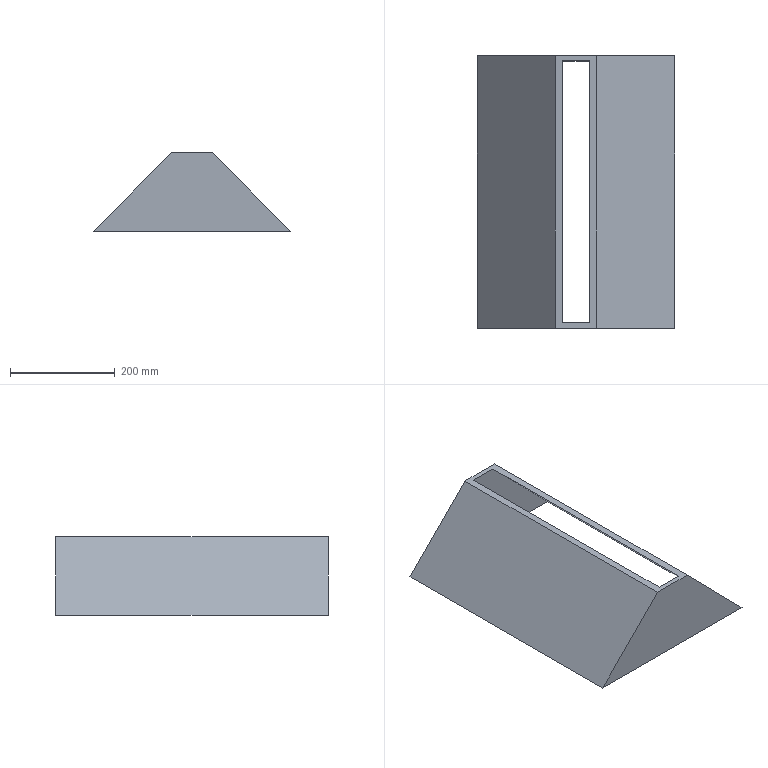Part | SolidWorks | features Extrusion 1, MirrorPattern 1, Shell 1 | 1 solid | 10 faces | box 376 x 520 x 150 mm | volume 2791226 mm3 | plane 10
STEP:
#1=CARTESIAN_POINT('',(-40.,0.,0.));
#2=VERTEX_POINT('',#1);
#3=CARTESIAN_POINT('',(40.,0.,0.));
#4=VERTEX_POINT('',#3);
#5=CARTESIAN_POINT('',(0.,0.,0.));
#6=DIRECTION('',(1.,0.,0.));
#7=VECTOR('',#6,1000.);
#8=LINE('',#5,#7);
#9=EDGE_CURVE('',#2,#4,#8,.T.);
#10=ORIENTED_EDGE('',*,*,#9,.T.);
#11=CARTESIAN_POINT('',(40.,520.,0.));
#12=VERTEX_POINT('',#11);
#13=CARTESIAN_POINT('',(40.,520.,0.));
#14=DIRECTION('',(0.,-1.,0.));
#15=VECTOR('',#14,1000.);
#16=LINE('',#13,#15);
#17=EDGE_CURVE('',#12,#4,#16,.T.);
#18=ORIENTED_EDGE('',*,*,#17,.F.);
#19=CARTESIAN_POINT('',(-40.,520.,0.));
#20=VERTEX_POINT('',#19);
#21=CARTESIAN_POINT('',(0.,520.,0.));
#22=DIRECTION('',(1.,0.,0.));
#23=VECTOR('',#22,1000.);
#24=LINE('',#21,#23);
#25=EDGE_CURVE('',#20,#12,#24,.T.);
#26=ORIENTED_EDGE('',*,*,#25,.F.);
#27=CARTESIAN_POINT('',(-40.,520.,0.));
#28=DIRECTION('',(0.,-1.,0.));
#29=VECTOR('',#28,1000.);
#30=LINE('',#27,#29);
#31=EDGE_CURVE('',#20,#2,#30,.T.);
#32=ORIENTED_EDGE('',*,*,#31,.T.);
#33=EDGE_LOOP('',(#10,#18,#26,#32));
#34=FACE_OUTER_BOUND('',#33,.T.);
#35=CARTESIAN_POINT('',(-25.952,10.,0.));
#36=VERTEX_POINT('',#35);
#37=CARTESIAN_POINT('',(25.952,10.,0.));
#38=VERTEX_POINT('',#37);
#39=CARTESIAN_POINT('',(0.,10.,0.));
#40=DIRECTION('',(1.,0.,0.));
#41=VECTOR('',#40,1000.);
#42=LINE('',#39,#41);
#43=EDGE_CURVE('',#36,#38,#42,.T.);
#44=ORIENTED_EDGE('',*,*,#43,.F.);
#45=CARTESIAN_POINT('',(-25.952,510.,0.));
#46=VERTEX_POINT('',#45);
#47=CARTESIAN_POINT('',(-25.952,520.,0.));
#48=DIRECTION('',(0.,-1.,0.));
#49=VECTOR('',#48,1000.);
#50=LINE('',#47,#49);
#51=EDGE_CURVE('',#46,#36,#50,.T.);
#52=ORIENTED_EDGE('',*,*,#51,.F.);
#53=CARTESIAN_POINT('',(25.952,510.,0.));
#54=VERTEX_POINT('',#53);
#55=CARTESIAN_POINT('',(0.,510.,0.));
#56=DIRECTION('',(1.,0.,0.));
#57=VECTOR('',#56,1000.);
#58=LINE('',#55,#57);
#59=EDGE_CURVE('',#46,#54,#58,.T.);
#60=ORIENTED_EDGE('',*,*,#59,.T.);
#61=CARTESIAN_POINT('',(25.952,520.,0.));
#62=DIRECTION('',(0.,-1.,0.));
#63=VECTOR('',#62,1000.);
#64=LINE('',#61,#63);
#65=EDGE_CURVE('',#54,#38,#64,.T.);
#66=ORIENTED_EDGE('',*,*,#65,.T.);
#67=EDGE_LOOP('',(#44,#52,#60,#66));
#68=FACE_BOUND('',#67,.T.);
#69=CARTESIAN_POINT('',(0.,520.,0.));
#70=DIRECTION('',(0.,0.,-1.));
#71=DIRECTION('',(-1.,0.,0.));
#72=AXIS2_PLACEMENT_3D('',#69,#70,#71);
#73=PLANE('',#72);
#74=ADVANCED_FACE('',(#34,#68),#73,.F.);
#75=CARTESIAN_POINT('',(188.,0.,-150.));
#76=VERTEX_POINT('',#75);
#77=CARTESIAN_POINT('',(-188.,0.,-150.));
#78=VERTEX_POINT('',#77);
#79=CARTESIAN_POINT('',(188.,0.,-150.));
#80=DIRECTION('',(-1.,0.,0.));
#81=VECTOR('',#80,1000.);
#82=LINE('',#79,#81);
#83=EDGE_CURVE('',#76,#78,#82,.T.);
#84=ORIENTED_EDGE('',*,*,#83,.T.);
#85=CARTESIAN_POINT('',(-188.,520.,-150.));
#86=VERTEX_POINT('',#85);
#87=CARTESIAN_POINT('',(-188.,520.,-150.));
#88=DIRECTION('',(0.,-1.,0.));
#89=VECTOR('',#88,1000.);
#90=LINE('',#87,#89);
#91=EDGE_CURVE('',#86,#78,#90,.T.);
#92=ORIENTED_EDGE('',*,*,#91,.F.);
#93=CARTESIAN_POINT('',(188.,520.,-150.));
#94=VERTEX_POINT('',#93);
#95=CARTESIAN_POINT('',(188.,520.,-150.));
#96=DIRECTION('',(-1.,0.,0.));
#97=VECTOR('',#96,1000.);
#98=LINE('',#95,#97);
#99=EDGE_CURVE('',#94,#86,#98,.T.);
#100=ORIENTED_EDGE('',*,*,#99,.F.);
#101=CARTESIAN_POINT('',(188.,520.,-150.));
#102=DIRECTION('',(0.,-1.,0.));
#103=VECTOR('',#102,1000.);
#104=LINE('',#101,#103);
#105=EDGE_CURVE('',#94,#76,#104,.T.);
#106=ORIENTED_EDGE('',*,*,#105,.T.);
#107=EDGE_LOOP('',(#84,#92,#100,#106));
#108=FACE_OUTER_BOUND('',#107,.T.);
#109=CARTESIAN_POINT('',(173.952,10.,-150.));
#110=VERTEX_POINT('',#109);
#111=CARTESIAN_POINT('',(-173.952,10.,-150.));
#112=VERTEX_POINT('',#111);
#113=CARTESIAN_POINT('',(188.,10.,-150.));
#114=DIRECTION('',(-1.,0.,0.));
#115=VECTOR('',#114,1000.);
#116=LINE('',#113,#115);
#117=EDGE_CURVE('',#110,#112,#116,.T.);
#118=ORIENTED_EDGE('',*,*,#117,.F.);
#119=CARTESIAN_POINT('',(173.952,510.,-150.));
#120=VERTEX_POINT('',#119);
#121=CARTESIAN_POINT('',(173.952,520.,-150.));
#122=DIRECTION('',(0.,-1.,0.));
#123=VECTOR('',#122,1000.);
#124=LINE('',#121,#123);
#125=EDGE_CURVE('',#120,#110,#124,.T.);
#126=ORIENTED_EDGE('',*,*,#125,.F.);
#127=CARTESIAN_POINT('',(-173.952,510.,-150.));
#128=VERTEX_POINT('',#127);
#129=CARTESIAN_POINT('',(188.,510.,-150.));
#130=DIRECTION('',(-1.,0.,0.));
#131=VECTOR('',#130,1000.);
#132=LINE('',#129,#131);
#133=EDGE_CURVE('',#120,#128,#132,.T.);
#134=ORIENTED_EDGE('',*,*,#133,.T.);
#135=CARTESIAN_POINT('',(-173.952,520.,-150.));
#136=DIRECTION('',(0.,-1.,0.));
#137=VECTOR('',#136,1000.);
#138=LINE('',#135,#137);
#139=EDGE_CURVE('',#128,#112,#138,.T.);
#140=ORIENTED_EDGE('',*,*,#139,.T.);
#141=EDGE_LOOP('',(#118,#126,#134,#140));
#142=FACE_BOUND('',#141,.T.);
#143=CARTESIAN_POINT('',(188.,520.,-150.));
#144=DIRECTION('',(0.,0.,1.));
#145=DIRECTION('',(1.,0.,0.));
#146=AXIS2_PLACEMENT_3D('',#143,#144,#145);
#147=PLANE('',#146);
#148=ADVANCED_FACE('',(#108,#142),#147,.F.);
#149=CARTESIAN_POINT('',(40.,0.,0.));
#150=DIRECTION('',(0.7023,0.,-0.7118));
#151=VECTOR('',#150,1000.);
#152=LINE('',#149,#151);
#153=EDGE_CURVE('',#4,#76,#152,.T.);
#154=ORIENTED_EDGE('',*,*,#153,.T.);
#155=ORIENTED_EDGE('',*,*,#105,.F.);
#156=CARTESIAN_POINT('',(40.,520.,0.));
#157=DIRECTION('',(0.7023,0.,-0.7118));
#158=VECTOR('',#157,1000.);
#159=LINE('',#156,#158);
#160=EDGE_CURVE('',#12,#94,#159,.T.);
#161=ORIENTED_EDGE('',*,*,#160,.F.);
#162=ORIENTED_EDGE('',*,*,#17,.T.);
#163=EDGE_LOOP('',(#154,#155,#161,#162));
#164=FACE_OUTER_BOUND('',#163,.T.);
#165=CARTESIAN_POINT('',(40.,520.,0.));
#166=DIRECTION('',(-0.7118,0.,-0.7023));
#167=DIRECTION('',(-0.7023,0.,0.7118));
#168=AXIS2_PLACEMENT_3D('',#165,#166,#167);
#169=PLANE('',#168);
#170=ADVANCED_FACE('',(#164),#169,.F.);
#171=ORIENTED_EDGE('',*,*,#99,.T.);
#172=CARTESIAN_POINT('',(-40.,520.,0.));
#173=DIRECTION('',(-0.7023,0.,-0.7118));
#174=VECTOR('',#173,1000.);
#175=LINE('',#172,#174);
#176=EDGE_CURVE('',#20,#86,#175,.T.);
#177=ORIENTED_EDGE('',*,*,#176,.F.);
#178=ORIENTED_EDGE('',*,*,#25,.T.);
#179=ORIENTED_EDGE('',*,*,#160,.T.);
#180=EDGE_LOOP('',(#171,#177,#178,#179));
#181=FACE_OUTER_BOUND('',#180,.T.);
#182=CARTESIAN_POINT('',(0.,520.,0.));
#183=DIRECTION('',(0.,1.,0.));
#184=DIRECTION('',(0.,0.,1.));
#185=AXIS2_PLACEMENT_3D('',#182,#183,#184);
#186=PLANE('',#185);
#187=ADVANCED_FACE('',(#181),#186,.T.);
#188=ORIENTED_EDGE('',*,*,#9,.F.);
#189=CARTESIAN_POINT('',(-40.,0.,0.));
#190=DIRECTION('',(-0.7023,0.,-0.7118));
#191=VECTOR('',#190,1000.);
#192=LINE('',#189,#191);
#193=EDGE_CURVE('',#2,#78,#192,.T.);
#194=ORIENTED_EDGE('',*,*,#193,.T.);
#195=ORIENTED_EDGE('',*,*,#83,.F.);
#196=ORIENTED_EDGE('',*,*,#153,.F.);
#197=EDGE_LOOP('',(#188,#194,#195,#196));
#198=FACE_OUTER_BOUND('',#197,.T.);
#199=CARTESIAN_POINT('',(0.,0.,0.));
#200=DIRECTION('',(0.,1.,0.));
#201=DIRECTION('',(0.,0.,1.));
#202=AXIS2_PLACEMENT_3D('',#199,#200,#201);
#203=PLANE('',#202);
#204=ADVANCED_FACE('',(#198),#203,.F.);
#205=ORIENTED_EDGE('',*,*,#193,.F.);
#206=ORIENTED_EDGE('',*,*,#31,.F.);
#207=ORIENTED_EDGE('',*,*,#176,.T.);
#208=ORIENTED_EDGE('',*,*,#91,.T.);
#209=EDGE_LOOP('',(#205,#206,#207,#208));
#210=FACE_OUTER_BOUND('',#209,.T.);
#211=CARTESIAN_POINT('',(-40.,520.,0.));
#212=DIRECTION('',(-0.7118,0.,0.7023));
#213=DIRECTION('',(0.7023,0.,0.7118));
#214=AXIS2_PLACEMENT_3D('',#211,#212,#213);
#215=PLANE('',#214);
#216=ADVANCED_FACE('',(#210),#215,.T.);
#217=CARTESIAN_POINT('',(32.882,10.,-7.023));
#218=DIRECTION('',(0.7023,0.,-0.7118));
#219=VECTOR('',#218,1000.);
#220=LINE('',#217,#219);
#221=EDGE_CURVE('',#38,#110,#220,.T.);
#222=ORIENTED_EDGE('',*,*,#221,.F.);
#223=ORIENTED_EDGE('',*,*,#65,.F.);
#224=CARTESIAN_POINT('',(32.882,510.,-7.023));
#225=DIRECTION('',(0.7023,0.,-0.7118));
#226=VECTOR('',#225,1000.);
#227=LINE('',#224,#226);
#228=EDGE_CURVE('',#54,#120,#227,.T.);
#229=ORIENTED_EDGE('',*,*,#228,.T.);
#230=ORIENTED_EDGE('',*,*,#125,.T.);
#231=EDGE_LOOP('',(#222,#223,#229,#230));
#232=FACE_OUTER_BOUND('',#231,.T.);
#233=CARTESIAN_POINT('',(32.882,520.,-7.023));
#234=DIRECTION('',(-0.7118,0.,-0.7023));
#235=DIRECTION('',(-0.7023,0.,0.7118));
#236=AXIS2_PLACEMENT_3D('',#233,#234,#235);
#237=PLANE('',#236);
#238=ADVANCED_FACE('',(#232),#237,.T.);
#239=ORIENTED_EDGE('',*,*,#133,.F.);
#240=ORIENTED_EDGE('',*,*,#228,.F.);
#241=ORIENTED_EDGE('',*,*,#59,.F.);
#242=CARTESIAN_POINT('',(-32.882,510.,-7.023));
#243=DIRECTION('',(-0.7023,0.,-0.7118));
#244=VECTOR('',#243,1000.);
#245=LINE('',#242,#244);
#246=EDGE_CURVE('',#46,#128,#245,.T.);
#247=ORIENTED_EDGE('',*,*,#246,.T.);
#248=EDGE_LOOP('',(#239,#240,#241,#247));
#249=FACE_OUTER_BOUND('',#248,.T.);
#250=CARTESIAN_POINT('',(0.,510.,0.));
#251=DIRECTION('',(0.,1.,0.));
#252=DIRECTION('',(0.,0.,1.));
#253=AXIS2_PLACEMENT_3D('',#250,#251,#252);
#254=PLANE('',#253);
#255=ADVANCED_FACE('',(#249),#254,.F.);
#256=ORIENTED_EDGE('',*,*,#43,.T.);
#257=ORIENTED_EDGE('',*,*,#221,.T.);
#258=ORIENTED_EDGE('',*,*,#117,.T.);
#259=CARTESIAN_POINT('',(-32.882,10.,-7.023));
#260=DIRECTION('',(-0.7023,0.,-0.7118));
#261=VECTOR('',#260,1000.);
#262=LINE('',#259,#261);
#263=EDGE_CURVE('',#36,#112,#262,.T.);
#264=ORIENTED_EDGE('',*,*,#263,.F.);
#265=EDGE_LOOP('',(#256,#257,#258,#264));
#266=FACE_OUTER_BOUND('',#265,.T.);
#267=CARTESIAN_POINT('',(0.,10.,0.));
#268=DIRECTION('',(0.,1.,0.));
#269=DIRECTION('',(0.,0.,1.));
#270=AXIS2_PLACEMENT_3D('',#267,#268,#269);
#271=PLANE('',#270);
#272=ADVANCED_FACE('',(#266),#271,.T.);
#273=ORIENTED_EDGE('',*,*,#263,.T.);
#274=ORIENTED_EDGE('',*,*,#139,.F.);
#275=ORIENTED_EDGE('',*,*,#246,.F.);
#276=ORIENTED_EDGE('',*,*,#51,.T.);
#277=EDGE_LOOP('',(#273,#274,#275,#276));
#278=FACE_OUTER_BOUND('',#277,.T.);
#279=CARTESIAN_POINT('',(-32.882,520.,-7.023));
#280=DIRECTION('',(-0.7118,0.,0.7023));
#281=DIRECTION('',(0.7023,0.,0.7118));
#282=AXIS2_PLACEMENT_3D('',#279,#280,#281);
#283=PLANE('',#282);
#284=ADVANCED_FACE('',(#278),#283,.F.);
#285=CLOSED_SHELL('',(#74,#148,#170,#187,#204,#216,#238,#255,#272,#284));
#286=MANIFOLD_SOLID_BREP('',#285);
#287=CARTESIAN_POINT('',(0.,0.,0.));
#288=DIRECTION('',(0.,0.,1.));
#289=DIRECTION('',(1.,0.,0.));
#290=AXIS2_PLACEMENT_3D('',#287,#288,#289);
#291=(LENGTH_UNIT()NAMED_UNIT(*)SI_UNIT(.MILLI.,.METRE.));
#292=UNCERTAINTY_MEASURE_WITH_UNIT(LENGTH_MEASURE(0.00001),#291,'','');
#293=(NAMED_UNIT(*)PLANE_ANGLE_UNIT()SI_UNIT($,.RADIAN.));
#294=(NAMED_UNIT(*)SI_UNIT($,.STERADIAN.)SOLID_ANGLE_UNIT());
#295=(GEOMETRIC_REPRESENTATION_CONTEXT(3)GLOBAL_UNCERTAINTY_ASSIGNED_CONTEXT((#292))GLOBAL_UNIT_ASSIGNED_CONTEXT((#291,#293,#294))REPRESENTATION_CONTEXT('',''));
#296=ADVANCED_BREP_SHAPE_REPRESENTATION('',(#286,#290),#295);